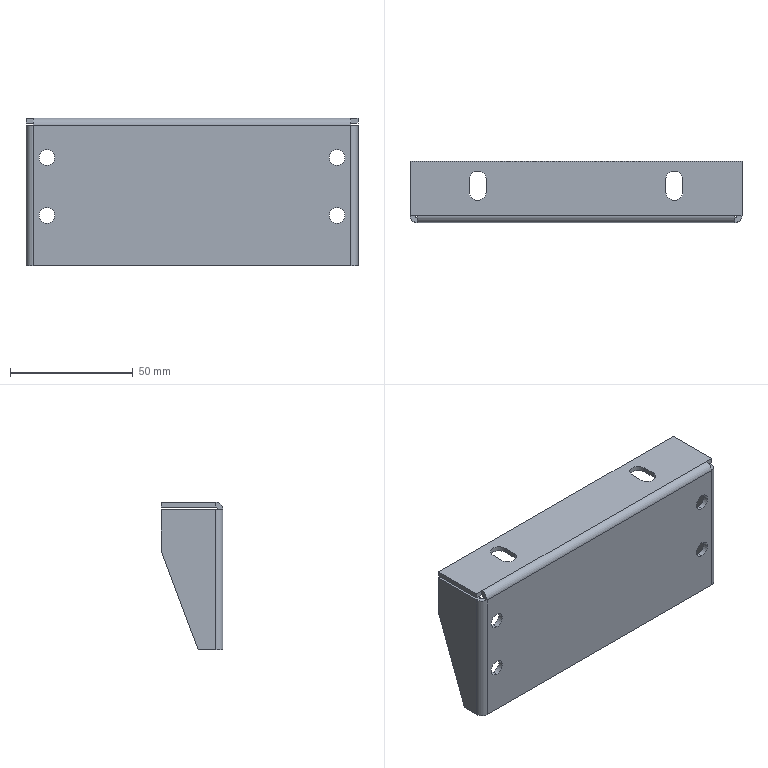Part | SolidWorks | features ICE 5, SMBaseFlange 2, EdgeFlange 1, FlatPattern 1, LPattern 1, SheetMetal 1 | 1 solid | 50 faces | box 135 x 25 x 60 mm | volume 25438 mm3 | plane 32 | cylinder 18 | commonest cylinder face diameters 6.4 x8 7 x4 2 x3 6 x3
STEP:
#1=CARTESIAN_POINT('',(158.643,39.897,40.8));
#2=VERTEX_POINT('',#1);
#3=CARTESIAN_POINT('',(158.643,39.897,47.2));
#4=VERTEX_POINT('',#3);
#5=CARTESIAN_POINT('',(158.643,39.897,44.));
#6=DIRECTION('',(0.,1.,0.));
#7=DIRECTION('',(0.,0.,1.));
#8=AXIS2_PLACEMENT_3D('',#5,#6,#7);
#9=CIRCLE('',#8,3.2);
#10=EDGE_CURVE('',#2,#4,#9,.T.);
#11=ORIENTED_EDGE('',*,*,#10,.T.);
#12=CARTESIAN_POINT('',(158.643,37.897,47.2));
#13=VERTEX_POINT('',#12);
#14=CARTESIAN_POINT('',(158.643,47.897,47.2));
#15=DIRECTION('',(0.,-1.,0.));
#16=VECTOR('',#15,1000.);
#17=LINE('',#14,#16);
#18=EDGE_CURVE('',#4,#13,#17,.T.);
#19=ORIENTED_EDGE('',*,*,#18,.T.);
#20=CARTESIAN_POINT('',(158.643,37.897,40.8));
#21=VERTEX_POINT('',#20);
#22=CARTESIAN_POINT('',(158.643,37.897,44.));
#23=DIRECTION('',(0.,-1.,0.));
#24=DIRECTION('',(0.,0.,-1.));
#25=AXIS2_PLACEMENT_3D('',#22,#23,#24);
#26=CIRCLE('',#25,3.2);
#27=EDGE_CURVE('',#13,#21,#26,.T.);
#28=ORIENTED_EDGE('',*,*,#27,.T.);
#29=CARTESIAN_POINT('',(158.643,47.897,40.8));
#30=DIRECTION('',(0.,-1.,0.));
#31=VECTOR('',#30,1000.);
#32=LINE('',#29,#31);
#33=EDGE_CURVE('',#2,#21,#32,.T.);
#34=ORIENTED_EDGE('',*,*,#33,.F.);
#35=EDGE_LOOP('',(#11,#19,#28,#34));
#36=FACE_OUTER_BOUND('',#35,.T.);
#37=CARTESIAN_POINT('',(158.643,47.897,44.));
#38=DIRECTION('',(0.,-1.,0.));
#39=DIRECTION('',(0.,0.,-1.));
#40=AXIS2_PLACEMENT_3D('',#37,#38,#39);
#41=CYLINDRICAL_SURFACE('',#40,3.2);
#42=ADVANCED_FACE('',(#36),#41,.F.);
#43=CARTESIAN_POINT('',(40.643,39.897,40.8));
#44=VERTEX_POINT('',#43);
#45=CARTESIAN_POINT('',(40.643,39.897,47.2));
#46=VERTEX_POINT('',#45);
#47=CARTESIAN_POINT('',(40.643,39.897,44.));
#48=DIRECTION('',(0.,1.,0.));
#49=DIRECTION('',(0.,0.,1.));
#50=AXIS2_PLACEMENT_3D('',#47,#48,#49);
#51=CIRCLE('',#50,3.2);
#52=EDGE_CURVE('',#44,#46,#51,.T.);
#53=ORIENTED_EDGE('',*,*,#52,.T.);
#54=CARTESIAN_POINT('',(40.643,37.897,47.2));
#55=VERTEX_POINT('',#54);
#56=CARTESIAN_POINT('',(40.643,47.897,47.2));
#57=DIRECTION('',(0.,-1.,0.));
#58=VECTOR('',#57,1000.);
#59=LINE('',#56,#58);
#60=EDGE_CURVE('',#46,#55,#59,.T.);
#61=ORIENTED_EDGE('',*,*,#60,.T.);
#62=CARTESIAN_POINT('',(40.643,37.897,40.8));
#63=VERTEX_POINT('',#62);
#64=CARTESIAN_POINT('',(40.643,37.897,44.));
#65=DIRECTION('',(0.,-1.,0.));
#66=DIRECTION('',(0.,0.,-1.));
#67=AXIS2_PLACEMENT_3D('',#64,#65,#66);
#68=CIRCLE('',#67,3.2);
#69=EDGE_CURVE('',#55,#63,#68,.T.);
#70=ORIENTED_EDGE('',*,*,#69,.T.);
#71=CARTESIAN_POINT('',(40.643,47.897,40.8));
#72=DIRECTION('',(0.,-1.,0.));
#73=VECTOR('',#72,1000.);
#74=LINE('',#71,#73);
#75=EDGE_CURVE('',#44,#63,#74,.T.);
#76=ORIENTED_EDGE('',*,*,#75,.F.);
#77=EDGE_LOOP('',(#53,#61,#70,#76));
#78=FACE_OUTER_BOUND('',#77,.T.);
#79=CARTESIAN_POINT('',(40.643,47.897,44.));
#80=DIRECTION('',(0.,-1.,0.));
#81=DIRECTION('',(0.,0.,-1.));
#82=AXIS2_PLACEMENT_3D('',#79,#80,#81);
#83=CYLINDRICAL_SURFACE('',#82,3.2);
#84=ADVANCED_FACE('',(#78),#83,.F.);
#85=CARTESIAN_POINT('',(40.643,39.897,17.3));
#86=VERTEX_POINT('',#85);
#87=CARTESIAN_POINT('',(40.643,39.897,23.7));
#88=VERTEX_POINT('',#87);
#89=CARTESIAN_POINT('',(40.643,39.897,20.5));
#90=DIRECTION('',(0.,1.,0.));
#91=DIRECTION('',(0.,0.,1.));
#92=AXIS2_PLACEMENT_3D('',#89,#90,#91);
#93=CIRCLE('',#92,3.2);
#94=EDGE_CURVE('',#86,#88,#93,.T.);
#95=ORIENTED_EDGE('',*,*,#94,.T.);
#96=CARTESIAN_POINT('',(40.643,37.897,23.7));
#97=VERTEX_POINT('',#96);
#98=CARTESIAN_POINT('',(40.643,47.897,23.7));
#99=DIRECTION('',(0.,-1.,0.));
#100=VECTOR('',#99,1000.);
#101=LINE('',#98,#100);
#102=EDGE_CURVE('',#88,#97,#101,.T.);
#103=ORIENTED_EDGE('',*,*,#102,.T.);
#104=CARTESIAN_POINT('',(40.643,37.897,17.3));
#105=VERTEX_POINT('',#104);
#106=CARTESIAN_POINT('',(40.643,37.897,20.5));
#107=DIRECTION('',(0.,-1.,0.));
#108=DIRECTION('',(0.,0.,-1.));
#109=AXIS2_PLACEMENT_3D('',#106,#107,#108);
#110=CIRCLE('',#109,3.2);
#111=EDGE_CURVE('',#97,#105,#110,.T.);
#112=ORIENTED_EDGE('',*,*,#111,.T.);
#113=CARTESIAN_POINT('',(40.643,47.897,17.3));
#114=DIRECTION('',(0.,-1.,0.));
#115=VECTOR('',#114,1000.);
#116=LINE('',#113,#115);
#117=EDGE_CURVE('',#86,#105,#116,.T.);
#118=ORIENTED_EDGE('',*,*,#117,.F.);
#119=EDGE_LOOP('',(#95,#103,#112,#118));
#120=FACE_OUTER_BOUND('',#119,.T.);
#121=CARTESIAN_POINT('',(40.643,47.897,20.5));
#122=DIRECTION('',(0.,-1.,0.));
#123=DIRECTION('',(0.,0.,-1.));
#124=AXIS2_PLACEMENT_3D('',#121,#122,#123);
#125=CYLINDRICAL_SURFACE('',#124,3.2);
#126=ADVANCED_FACE('',(#120),#125,.F.);
#127=CARTESIAN_POINT('',(158.643,39.897,17.3));
#128=VERTEX_POINT('',#127);
#129=CARTESIAN_POINT('',(158.643,39.897,23.7));
#130=VERTEX_POINT('',#129);
#131=CARTESIAN_POINT('',(158.643,39.897,20.5));
#132=DIRECTION('',(0.,1.,0.));
#133=DIRECTION('',(0.,0.,1.));
#134=AXIS2_PLACEMENT_3D('',#131,#132,#133);
#135=CIRCLE('',#134,3.2);
#136=EDGE_CURVE('',#128,#130,#135,.T.);
#137=ORIENTED_EDGE('',*,*,#136,.T.);
#138=CARTESIAN_POINT('',(158.643,37.897,23.7));
#139=VERTEX_POINT('',#138);
#140=CARTESIAN_POINT('',(158.643,47.897,23.7));
#141=DIRECTION('',(0.,-1.,0.));
#142=VECTOR('',#141,1000.);
#143=LINE('',#140,#142);
#144=EDGE_CURVE('',#130,#139,#143,.T.);
#145=ORIENTED_EDGE('',*,*,#144,.T.);
#146=CARTESIAN_POINT('',(158.643,37.897,17.3));
#147=VERTEX_POINT('',#146);
#148=CARTESIAN_POINT('',(158.643,37.897,20.5));
#149=DIRECTION('',(0.,-1.,0.));
#150=DIRECTION('',(0.,0.,-1.));
#151=AXIS2_PLACEMENT_3D('',#148,#149,#150);
#152=CIRCLE('',#151,3.2);
#153=EDGE_CURVE('',#139,#147,#152,.T.);
#154=ORIENTED_EDGE('',*,*,#153,.T.);
#155=CARTESIAN_POINT('',(158.643,47.897,17.3));
#156=DIRECTION('',(0.,-1.,0.));
#157=VECTOR('',#156,1000.);
#158=LINE('',#155,#157);
#159=EDGE_CURVE('',#128,#147,#158,.T.);
#160=ORIENTED_EDGE('',*,*,#159,.F.);
#161=EDGE_LOOP('',(#137,#145,#154,#160));
#162=FACE_OUTER_BOUND('',#161,.T.);
#163=CARTESIAN_POINT('',(158.643,47.897,20.5));
#164=DIRECTION('',(0.,-1.,0.));
#165=DIRECTION('',(0.,0.,-1.));
#166=AXIS2_PLACEMENT_3D('',#163,#164,#165);
#167=CYLINDRICAL_SURFACE('',#166,3.2);
#168=ADVANCED_FACE('',(#162),#167,.F.);
#169=CARTESIAN_POINT('',(34.143,62.897,57.));
#170=VERTEX_POINT('',#169);
#171=CARTESIAN_POINT('',(34.143,62.897,40.));
#172=VERTEX_POINT('',#171);
#173=CARTESIAN_POINT('',(34.143,62.897,60.));
#174=DIRECTION('',(0.,0.,-1.));
#175=VECTOR('',#174,1000.);
#176=LINE('',#173,#175);
#177=EDGE_CURVE('',#170,#172,#176,.T.);
#178=ORIENTED_EDGE('',*,*,#177,.F.);
#179=CARTESIAN_POINT('',(34.143,40.897,57.));
#180=VERTEX_POINT('',#179);
#181=CARTESIAN_POINT('',(34.143,62.897,57.));
#182=DIRECTION('',(0.,-1.,0.));
#183=VECTOR('',#182,1000.);
#184=LINE('',#181,#183);
#185=EDGE_CURVE('',#170,#180,#184,.T.);
#186=ORIENTED_EDGE('',*,*,#185,.T.);
#187=CARTESIAN_POINT('',(34.143,40.897,0.));
#188=VERTEX_POINT('',#187);
#189=CARTESIAN_POINT('',(34.143,40.897,60.));
#190=DIRECTION('',(0.,0.,-1.));
#191=VECTOR('',#190,1000.);
#192=LINE('',#189,#191);
#193=EDGE_CURVE('',#180,#188,#192,.T.);
#194=ORIENTED_EDGE('',*,*,#193,.T.);
#195=CARTESIAN_POINT('',(34.143,47.897,0.));
#196=VERTEX_POINT('',#195);
#197=CARTESIAN_POINT('',(34.143,62.897,0.));
#198=DIRECTION('',(0.,-1.,0.));
#199=VECTOR('',#198,1000.);
#200=LINE('',#197,#199);
#201=EDGE_CURVE('',#196,#188,#200,.T.);
#202=ORIENTED_EDGE('',*,*,#201,.F.);
#203=CARTESIAN_POINT('',(34.143,69.472,57.534));
#204=DIRECTION('',(0.,-0.3511,-0.9363));
#205=VECTOR('',#204,1000.);
#206=LINE('',#203,#205);
#207=EDGE_CURVE('',#172,#196,#206,.T.);
#208=ORIENTED_EDGE('',*,*,#207,.F.);
#209=EDGE_LOOP('',(#178,#186,#194,#202,#208));
#210=FACE_OUTER_BOUND('',#209,.T.);
#211=CARTESIAN_POINT('',(34.143,62.897,60.));
#212=DIRECTION('',(1.,0.,0.));
#213=DIRECTION('',(0.,0.,-1.));
#214=AXIS2_PLACEMENT_3D('',#211,#212,#213);
#215=PLANE('',#214);
#216=ADVANCED_FACE('',(#210),#215,.T.);
#217=CARTESIAN_POINT('',(32.143,62.897,57.));
#218=VERTEX_POINT('',#217);
#219=CARTESIAN_POINT('',(32.143,62.897,40.));
#220=VERTEX_POINT('',#219);
#221=CARTESIAN_POINT('',(32.143,62.897,60.));
#222=DIRECTION('',(0.,0.,-1.));
#223=VECTOR('',#222,1000.);
#224=LINE('',#221,#223);
#225=EDGE_CURVE('',#218,#220,#224,.T.);
#226=ORIENTED_EDGE('',*,*,#225,.F.);
#227=CARTESIAN_POINT('',(32.143,62.897,57.));
#228=DIRECTION('',(1.,0.,0.));
#229=VECTOR('',#228,1000.);
#230=LINE('',#227,#229);
#231=EDGE_CURVE('',#218,#170,#230,.T.);
#232=ORIENTED_EDGE('',*,*,#231,.T.);
#233=ORIENTED_EDGE('',*,*,#177,.T.);
#234=CARTESIAN_POINT('',(34.143,62.897,40.));
#235=DIRECTION('',(-1.,0.,0.));
#236=VECTOR('',#235,1000.);
#237=LINE('',#234,#236);
#238=EDGE_CURVE('',#172,#220,#237,.T.);
#239=ORIENTED_EDGE('',*,*,#238,.T.);
#240=EDGE_LOOP('',(#226,#232,#233,#239));
#241=FACE_OUTER_BOUND('',#240,.T.);
#242=CARTESIAN_POINT('',(32.143,62.897,60.));
#243=DIRECTION('',(0.,1.,0.));
#244=DIRECTION('',(0.,0.,1.));
#245=AXIS2_PLACEMENT_3D('',#242,#243,#244);
#246=PLANE('',#245);
#247=ADVANCED_FACE('',(#241),#246,.T.);
#248=CARTESIAN_POINT('',(32.143,40.897,57.));
#249=VERTEX_POINT('',#248);
#250=CARTESIAN_POINT('',(32.143,62.897,57.));
#251=DIRECTION('',(0.,-1.,0.));
#252=VECTOR('',#251,1000.);
#253=LINE('',#250,#252);
#254=EDGE_CURVE('',#218,#249,#253,.T.);
#255=ORIENTED_EDGE('',*,*,#254,.F.);
#256=ORIENTED_EDGE('',*,*,#225,.T.);
#257=CARTESIAN_POINT('',(32.143,47.897,0.));
#258=VERTEX_POINT('',#257);
#259=CARTESIAN_POINT('',(32.143,69.472,57.534));
#260=DIRECTION('',(0.,-0.3511,-0.9363));
#261=VECTOR('',#260,1000.);
#262=LINE('',#259,#261);
#263=EDGE_CURVE('',#220,#258,#262,.T.);
#264=ORIENTED_EDGE('',*,*,#263,.T.);
#265=CARTESIAN_POINT('',(32.143,40.897,0.));
#266=VERTEX_POINT('',#265);
#267=CARTESIAN_POINT('',(32.143,62.897,0.));
#268=DIRECTION('',(0.,-1.,0.));
#269=VECTOR('',#268,1000.);
#270=LINE('',#267,#269);
#271=EDGE_CURVE('',#258,#266,#270,.T.);
#272=ORIENTED_EDGE('',*,*,#271,.T.);
#273=CARTESIAN_POINT('',(32.143,40.897,60.));
#274=DIRECTION('',(0.,0.,-1.));
#275=VECTOR('',#274,1000.);
#276=LINE('',#273,#275);
#277=EDGE_CURVE('',#249,#266,#276,.T.);
#278=ORIENTED_EDGE('',*,*,#277,.F.);
#279=EDGE_LOOP('',(#255,#256,#264,#272,#278));
#280=FACE_OUTER_BOUND('',#279,.T.);
#281=CARTESIAN_POINT('',(32.143,62.897,60.));
#282=DIRECTION('',(1.,0.,0.));
#283=DIRECTION('',(0.,0.,-1.));
#284=AXIS2_PLACEMENT_3D('',#281,#282,#283);
#285=PLANE('',#284);
#286=ADVANCED_FACE('',(#280),#285,.F.);
#287=CARTESIAN_POINT('',(167.143,40.897,57.));
#288=VERTEX_POINT('',#287);
#289=CARTESIAN_POINT('',(167.143,62.897,57.));
#290=VERTEX_POINT('',#289);
#291=CARTESIAN_POINT('',(167.143,62.897,57.));
#292=DIRECTION('',(0.,1.,0.));
#293=VECTOR('',#292,1000.);
#294=LINE('',#291,#293);
#295=EDGE_CURVE('',#288,#290,#294,.T.);
#296=ORIENTED_EDGE('',*,*,#295,.F.);
#297=CARTESIAN_POINT('',(167.143,40.897,0.));
#298=VERTEX_POINT('',#297);
#299=CARTESIAN_POINT('',(167.143,40.897,60.));
#300=DIRECTION('',(0.,0.,-1.));
#301=VECTOR('',#300,1000.);
#302=LINE('',#299,#301);
#303=EDGE_CURVE('',#288,#298,#302,.T.);
#304=ORIENTED_EDGE('',*,*,#303,.T.);
#305=CARTESIAN_POINT('',(167.143,47.897,0.));
#306=VERTEX_POINT('',#305);
#307=CARTESIAN_POINT('',(167.143,37.897,0.));
#308=DIRECTION('',(0.,1.,0.));
#309=VECTOR('',#308,1000.);
#310=LINE('',#307,#309);
#311=EDGE_CURVE('',#298,#306,#310,.T.);
#312=ORIENTED_EDGE('',*,*,#311,.T.);
#313=CARTESIAN_POINT('',(167.143,62.897,40.));
#314=VERTEX_POINT('',#313);
#315=CARTESIAN_POINT('',(167.143,66.39,49.315));
#316=DIRECTION('',(0.,0.3511,0.9363));
#317=VECTOR('',#316,1000.);
#318=LINE('',#315,#317);
#319=EDGE_CURVE('',#306,#314,#318,.T.);
#320=ORIENTED_EDGE('',*,*,#319,.T.);
#321=CARTESIAN_POINT('',(167.143,62.897,60.));
#322=DIRECTION('',(0.,0.,-1.));
#323=VECTOR('',#322,1000.);
#324=LINE('',#321,#323);
#325=EDGE_CURVE('',#290,#314,#324,.T.);
#326=ORIENTED_EDGE('',*,*,#325,.F.);
#327=EDGE_LOOP('',(#296,#304,#312,#320,#326));
#328=FACE_OUTER_BOUND('',#327,.T.);
#329=CARTESIAN_POINT('',(167.143,37.897,60.));
#330=DIRECTION('',(-1.,0.,0.));
#331=DIRECTION('',(0.,0.,1.));
#332=AXIS2_PLACEMENT_3D('',#329,#330,#331);
#333=PLANE('',#332);
#334=ADVANCED_FACE('',(#328),#333,.F.);
#335=CARTESIAN_POINT('',(165.143,62.897,57.));
#336=VERTEX_POINT('',#335);
#337=CARTESIAN_POINT('',(165.143,62.897,40.));
#338=VERTEX_POINT('',#337);
#339=CARTESIAN_POINT('',(165.143,62.897,60.));
#340=DIRECTION('',(0.,0.,-1.));
#341=VECTOR('',#340,1000.);
#342=LINE('',#339,#341);
#343=EDGE_CURVE('',#336,#338,#342,.T.);
#344=ORIENTED_EDGE('',*,*,#343,.F.);
#345=CARTESIAN_POINT('',(167.143,62.897,57.));
#346=DIRECTION('',(-1.,0.,0.));
#347=VECTOR('',#346,1000.);
#348=LINE('',#345,#347);
#349=EDGE_CURVE('',#290,#336,#348,.T.);
#350=ORIENTED_EDGE('',*,*,#349,.F.);
#351=ORIENTED_EDGE('',*,*,#325,.T.);
#352=CARTESIAN_POINT('',(165.143,62.897,40.));
#353=DIRECTION('',(1.,0.,0.));
#354=VECTOR('',#353,1000.);
#355=LINE('',#352,#354);
#356=EDGE_CURVE('',#338,#314,#355,.T.);
#357=ORIENTED_EDGE('',*,*,#356,.F.);
#358=EDGE_LOOP('',(#344,#350,#351,#357));
#359=FACE_OUTER_BOUND('',#358,.T.);
#360=CARTESIAN_POINT('',(165.143,62.897,60.));
#361=DIRECTION('',(0.,1.,0.));
#362=DIRECTION('',(0.,0.,1.));
#363=AXIS2_PLACEMENT_3D('',#360,#361,#362);
#364=PLANE('',#363);
#365=ADVANCED_FACE('',(#359),#364,.T.);
#366=CARTESIAN_POINT('',(165.143,40.897,57.));
#367=VERTEX_POINT('',#366);
#368=CARTESIAN_POINT('',(165.143,40.897,0.));
#369=VERTEX_POINT('',#368);
#370=CARTESIAN_POINT('',(165.143,40.897,60.));
#371=DIRECTION('',(0.,0.,-1.));
#372=VECTOR('',#371,1000.);
#373=LINE('',#370,#372);
#374=EDGE_CURVE('',#367,#369,#373,.T.);
#375=ORIENTED_EDGE('',*,*,#374,.F.);
#376=CARTESIAN_POINT('',(165.143,37.897,57.));
#377=DIRECTION('',(0.,1.,0.));
#378=VECTOR('',#377,1000.);
#379=LINE('',#376,#378);
#380=EDGE_CURVE('',#367,#336,#379,.T.);
#381=ORIENTED_EDGE('',*,*,#380,.T.);
#382=ORIENTED_EDGE('',*,*,#343,.T.);
#383=CARTESIAN_POINT('',(165.143,47.897,0.));
#384=VERTEX_POINT('',#383);
#385=CARTESIAN_POINT('',(165.143,66.39,49.315));
#386=DIRECTION('',(0.,0.3511,0.9363));
#387=VECTOR('',#386,1000.);
#388=LINE('',#385,#387);
#389=EDGE_CURVE('',#384,#338,#388,.T.);
#390=ORIENTED_EDGE('',*,*,#389,.F.);
#391=CARTESIAN_POINT('',(165.143,37.897,0.));
#392=DIRECTION('',(0.,1.,0.));
#393=VECTOR('',#392,1000.);
#394=LINE('',#391,#393);
#395=EDGE_CURVE('',#369,#384,#394,.T.);
#396=ORIENTED_EDGE('',*,*,#395,.F.);
#397=EDGE_LOOP('',(#375,#381,#382,#390,#396));
#398=FACE_OUTER_BOUND('',#397,.T.);
#399=CARTESIAN_POINT('',(165.143,37.897,60.));
#400=DIRECTION('',(-1.,0.,0.));
#401=DIRECTION('',(0.,0.,1.));
#402=AXIS2_PLACEMENT_3D('',#399,#400,#401);
#403=PLANE('',#402);
#404=ADVANCED_FACE('',(#398),#403,.T.);
#405=ORIENTED_EDGE('',*,*,#144,.F.);
#406=CARTESIAN_POINT('',(158.643,39.897,20.5));
#407=DIRECTION('',(0.,1.,0.));
#408=DIRECTION('',(0.,0.,1.));
#409=AXIS2_PLACEMENT_3D('',#406,#407,#408);
#410=CIRCLE('',#409,3.2);
#411=EDGE_CURVE('',#130,#128,#410,.T.);
#412=ORIENTED_EDGE('',*,*,#411,.T.);
#413=ORIENTED_EDGE('',*,*,#159,.T.);
#414=CARTESIAN_POINT('',(158.643,37.897,20.5));
#415=DIRECTION('',(0.,-1.,0.));
#416=DIRECTION('',(0.,0.,-1.));
#417=AXIS2_PLACEMENT_3D('',#414,#415,#416);
#418=CIRCLE('',#417,3.2);
#419=EDGE_CURVE('',#147,#139,#418,.T.);
#420=ORIENTED_EDGE('',*,*,#419,.T.);
#421=EDGE_LOOP('',(#405,#412,#413,#420));
#422=FACE_OUTER_BOUND('',#421,.T.);
#423=CARTESIAN_POINT('',(158.643,47.897,20.5));
#424=DIRECTION('',(0.,-1.,0.));
#425=DIRECTION('',(0.,0.,-1.));
#426=AXIS2_PLACEMENT_3D('',#423,#424,#425);
#427=CYLINDRICAL_SURFACE('',#426,3.2);
#428=ADVANCED_FACE('',(#422),#427,.F.);
#429=ORIENTED_EDGE('',*,*,#102,.F.);
#430=CARTESIAN_POINT('',(40.643,39.897,20.5));
#431=DIRECTION('',(0.,1.,0.));
#432=DIRECTION('',(0.,0.,1.));
#433=AXIS2_PLACEMENT_3D('',#430,#431,#432);
#434=CIRCLE('',#433,3.2);
#435=EDGE_CURVE('',#88,#86,#434,.T.);
#436=ORIENTED_EDGE('',*,*,#435,.T.);
#437=ORIENTED_EDGE('',*,*,#117,.T.);
#438=CARTESIAN_POINT('',(40.643,37.897,20.5));
#439=DIRECTION('',(0.,-1.,0.));
#440=DIRECTION('',(0.,0.,-1.));
#441=AXIS2_PLACEMENT_3D('',#438,#439,#440);
#442=CIRCLE('',#441,3.2);
#443=EDGE_CURVE('',#105,#97,#442,.T.);
#444=ORIENTED_EDGE('',*,*,#443,.T.);
#445=EDGE_LOOP('',(#429,#436,#437,#444));
#446=FACE_OUTER_BOUND('',#445,.T.);
#447=CARTESIAN_POINT('',(40.643,47.897,20.5));
#448=DIRECTION('',(0.,-1.,0.));
#449=DIRECTION('',(0.,0.,-1.));
#450=AXIS2_PLACEMENT_3D('',#447,#448,#449);
#451=CYLINDRICAL_SURFACE('',#450,3.2);
#452=ADVANCED_FACE('',(#446),#451,.F.);
#453=ORIENTED_EDGE('',*,*,#395,.T.);
#454=CARTESIAN_POINT('',(165.143,47.897,0.));
#455=DIRECTION('',(1.,0.,0.));
#456=VECTOR('',#455,1000.);
#457=LINE('',#454,#456);
#458=EDGE_CURVE('',#384,#306,#457,.T.);
#459=ORIENTED_EDGE('',*,*,#458,.T.);
#460=ORIENTED_EDGE('',*,*,#311,.F.);
#461=CARTESIAN_POINT('',(167.143,40.897,0.));
#462=DIRECTION('',(-1.,0.,0.));
#463=VECTOR('',#462,1000.);
#464=LINE('',#461,#463);
#465=EDGE_CURVE('',#298,#369,#464,.T.);
#466=ORIENTED_EDGE('',*,*,#465,.T.);
#467=EDGE_LOOP('',(#453,#459,#460,#466));
#468=FACE_OUTER_BOUND('',#467,.T.);
#469=CARTESIAN_POINT('',(164.143,39.897,0.));
#470=DIRECTION('',(0.,0.,-1.));
#471=DIRECTION('',(-1.,0.,0.));
#472=AXIS2_PLACEMENT_3D('',#469,#470,#471);
#473=PLANE('',#472);
#474=ADVANCED_FACE('',(#468),#473,.T.);
#475=CARTESIAN_POINT('',(34.143,47.897,0.));
#476=DIRECTION('',(-1.,0.,0.));
#477=VECTOR('',#476,1000.);
#478=LINE('',#475,#477);
#479=EDGE_CURVE('',#196,#258,#478,.T.);
#480=ORIENTED_EDGE('',*,*,#479,.F.);
#481=ORIENTED_EDGE('',*,*,#201,.T.);
#482=CARTESIAN_POINT('',(34.143,40.897,0.));
#483=DIRECTION('',(-1.,0.,0.));
#484=VECTOR('',#483,1000.);
#485=LINE('',#482,#484);
#486=EDGE_CURVE('',#188,#266,#485,.T.);
#487=ORIENTED_EDGE('',*,*,#486,.T.);
#488=ORIENTED_EDGE('',*,*,#271,.F.);
#489=EDGE_LOOP('',(#480,#481,#487,#488));
#490=FACE_OUTER_BOUND('',#489,.T.);
#491=CARTESIAN_POINT('',(164.143,40.897,0.));
#492=DIRECTION('',(0.,0.,1.));
#493=DIRECTION('',(1.,0.,0.));
#494=AXIS2_PLACEMENT_3D('',#491,#492,#493);
#495=PLANE('',#494);
#496=ADVANCED_FACE('',(#490),#495,.F.);
#497=ORIENTED_EDGE('',*,*,#193,.F.);
#498=CARTESIAN_POINT('',(35.143,39.897,57.));
#499=VERTEX_POINT('',#498);
#500=CARTESIAN_POINT('',(35.143,40.897,57.));
#501=DIRECTION('',(0.,0.,1.));
#502=DIRECTION('',(0.,-1.,0.));
#503=AXIS2_PLACEMENT_3D('',#500,#501,#502);
#504=CIRCLE('',#503,1.);
#505=EDGE_CURVE('',#180,#499,#504,.T.);
#506=ORIENTED_EDGE('',*,*,#505,.T.);
#507=CARTESIAN_POINT('',(35.143,39.897,0.));
#508=VERTEX_POINT('',#507);
#509=CARTESIAN_POINT('',(35.143,39.897,60.));
#510=DIRECTION('',(0.,0.,-1.));
#511=VECTOR('',#510,1000.);
#512=LINE('',#509,#511);
#513=EDGE_CURVE('',#499,#508,#512,.T.);
#514=ORIENTED_EDGE('',*,*,#513,.T.);
#515=CARTESIAN_POINT('',(35.143,40.897,0.));
#516=DIRECTION('',(0.,0.,1.));
#517=DIRECTION('',(1.,0.,0.));
#518=AXIS2_PLACEMENT_3D('',#515,#516,#517);
#519=CIRCLE('',#518,1.);
#520=EDGE_CURVE('',#188,#508,#519,.T.);
#521=ORIENTED_EDGE('',*,*,#520,.F.);
#522=EDGE_LOOP('',(#497,#506,#514,#521));
#523=FACE_OUTER_BOUND('',#522,.T.);
#524=CARTESIAN_POINT('',(35.143,40.897,60.));
#525=DIRECTION('',(0.,0.,-1.));
#526=DIRECTION('',(-1.,0.,0.));
#527=AXIS2_PLACEMENT_3D('',#524,#525,#526);
#528=CYLINDRICAL_SURFACE('',#527,1.);
#529=ADVANCED_FACE('',(#523),#528,.F.);
#530=CARTESIAN_POINT('',(164.143,39.897,57.));
#531=VERTEX_POINT('',#530);
#532=CARTESIAN_POINT('',(164.143,39.897,0.));
#533=VERTEX_POINT('',#532);
#534=CARTESIAN_POINT('',(164.143,39.897,60.));
#535=DIRECTION('',(0.,0.,-1.));
#536=VECTOR('',#535,1000.);
#537=LINE('',#534,#536);
#538=EDGE_CURVE('',#531,#533,#537,.T.);
#539=ORIENTED_EDGE('',*,*,#538,.F.);
#540=CARTESIAN_POINT('',(164.143,40.897,57.));
#541=DIRECTION('',(0.,0.,1.));
#542=DIRECTION('',(0.,-1.,0.));
#543=AXIS2_PLACEMENT_3D('',#540,#541,#542);
#544=CIRCLE('',#543,1.);
#545=EDGE_CURVE('',#531,#367,#544,.T.);
#546=ORIENTED_EDGE('',*,*,#545,.T.);
#547=ORIENTED_EDGE('',*,*,#374,.T.);
#548=CARTESIAN_POINT('',(164.143,40.897,0.));
#549=DIRECTION('',(0.,0.,1.));
#550=DIRECTION('',(1.,0.,0.));
#551=AXIS2_PLACEMENT_3D('',#548,#549,#550);
#552=CIRCLE('',#551,1.);
#553=EDGE_CURVE('',#533,#369,#552,.T.);
#554=ORIENTED_EDGE('',*,*,#553,.F.);
#555=EDGE_LOOP('',(#539,#546,#547,#554));
#556=FACE_OUTER_BOUND('',#555,.T.);
#557=CARTESIAN_POINT('',(164.143,40.897,60.));
#558=DIRECTION('',(0.,0.,-1.));
#559=DIRECTION('',(-1.,0.,0.));
#560=AXIS2_PLACEMENT_3D('',#557,#558,#559);
#561=CYLINDRICAL_SURFACE('',#560,1.);
#562=ADVANCED_FACE('',(#556),#561,.F.);
#563=CARTESIAN_POINT('',(164.143,37.897,57.));
#564=VERTEX_POINT('',#563);
#565=CARTESIAN_POINT('',(164.143,40.897,57.));
#566=DIRECTION('',(0.,0.,1.));
#567=DIRECTION('',(0.,-1.,0.));
#568=AXIS2_PLACEMENT_3D('',#565,#566,#567);
#569=CIRCLE('',#568,3.);
#570=EDGE_CURVE('',#564,#288,#569,.T.);
#571=ORIENTED_EDGE('',*,*,#570,.T.);
#572=CARTESIAN_POINT('',(167.143,40.897,57.));
#573=DIRECTION('',(-1.,0.,0.));
#574=VECTOR('',#573,1000.);
#575=LINE('',#572,#574);
#576=EDGE_CURVE('',#288,#367,#575,.T.);
#577=ORIENTED_EDGE('',*,*,#576,.T.);
#578=ORIENTED_EDGE('',*,*,#545,.F.);
#579=CARTESIAN_POINT('',(164.143,39.897,57.));
#580=DIRECTION('',(0.,-1.,0.));
#581=VECTOR('',#580,1000.);
#582=LINE('',#579,#581);
#583=EDGE_CURVE('',#531,#564,#582,.T.);
#584=ORIENTED_EDGE('',*,*,#583,.T.);
#585=EDGE_LOOP('',(#571,#577,#578,#584));
#586=FACE_OUTER_BOUND('',#585,.T.);
#587=CARTESIAN_POINT('',(164.143,40.897,57.));
#588=DIRECTION('',(0.,0.,1.));
#589=DIRECTION('',(0.,-1.,0.));
#590=AXIS2_PLACEMENT_3D('',#587,#588,#589);
#591=PLANE('',#590);
#592=ADVANCED_FACE('',(#586),#591,.T.);
#593=ORIENTED_EDGE('',*,*,#10,.F.);
#594=CARTESIAN_POINT('',(158.643,39.897,44.));
#595=DIRECTION('',(0.,1.,0.));
#596=DIRECTION('',(0.,0.,1.));
#597=AXIS2_PLACEMENT_3D('',#594,#595,#596);
#598=CIRCLE('',#597,3.2);
#599=EDGE_CURVE('',#4,#2,#598,.T.);
#600=ORIENTED_EDGE('',*,*,#599,.F.);
#601=EDGE_LOOP('',(#593,#600));
#602=FACE_BOUND('',#601,.T.);
#603=ORIENTED_EDGE('',*,*,#52,.F.);
#604=CARTESIAN_POINT('',(40.643,39.897,44.));
#605=DIRECTION('',(0.,1.,0.));
#606=DIRECTION('',(0.,0.,1.));
#607=AXIS2_PLACEMENT_3D('',#604,#605,#606);
#608=CIRCLE('',#607,3.2);
#609=EDGE_CURVE('',#46,#44,#608,.T.);
#610=ORIENTED_EDGE('',*,*,#609,.F.);
#611=EDGE_LOOP('',(#603,#610));
#612=FACE_BOUND('',#611,.T.);
#613=ORIENTED_EDGE('',*,*,#513,.F.);
#614=CARTESIAN_POINT('',(164.143,39.897,57.));
#615=DIRECTION('',(-1.,0.,0.));
#616=VECTOR('',#615,1000.);
#617=LINE('',#614,#616);
#618=EDGE_CURVE('',#531,#499,#617,.T.);
#619=ORIENTED_EDGE('',*,*,#618,.F.);
#620=ORIENTED_EDGE('',*,*,#538,.T.);
#621=CARTESIAN_POINT('',(32.143,39.897,0.));
#622=DIRECTION('',(1.,0.,0.));
#623=VECTOR('',#622,1000.);
#624=LINE('',#621,#623);
#625=EDGE_CURVE('',#508,#533,#624,.T.);
#626=ORIENTED_EDGE('',*,*,#625,.F.);
#627=EDGE_LOOP('',(#613,#619,#620,#626));
#628=FACE_OUTER_BOUND('',#627,.T.);
#629=ORIENTED_EDGE('',*,*,#94,.F.);
#630=ORIENTED_EDGE('',*,*,#435,.F.);
#631=EDGE_LOOP('',(#629,#630));
#632=FACE_BOUND('',#631,.T.);
#633=ORIENTED_EDGE('',*,*,#136,.F.);
#634=ORIENTED_EDGE('',*,*,#411,.F.);
#635=EDGE_LOOP('',(#633,#634));
#636=FACE_BOUND('',#635,.T.);
#637=CARTESIAN_POINT('',(32.143,39.897,60.));
#638=DIRECTION('',(0.,1.,0.));
#639=DIRECTION('',(0.,0.,1.));
#640=AXIS2_PLACEMENT_3D('',#637,#638,#639);
#641=PLANE('',#640);
#642=ADVANCED_FACE('',(#602,#612,#628,#632,#636),#641,.T.);
#643=CARTESIAN_POINT('',(158.643,37.897,44.));
#644=DIRECTION('',(0.,-1.,0.));
#645=DIRECTION('',(0.,0.,-1.));
#646=AXIS2_PLACEMENT_3D('',#643,#644,#645);
#647=CIRCLE('',#646,3.2);
#648=EDGE_CURVE('',#21,#13,#647,.T.);
#649=ORIENTED_EDGE('',*,*,#648,.F.);
#650=ORIENTED_EDGE('',*,*,#27,.F.);
#651=EDGE_LOOP('',(#649,#650));
#652=FACE_BOUND('',#651,.T.);
#653=CARTESIAN_POINT('',(40.643,37.897,44.));
#654=DIRECTION('',(0.,-1.,0.));
#655=DIRECTION('',(0.,0.,-1.));
#656=AXIS2_PLACEMENT_3D('',#653,#654,#655);
#657=CIRCLE('',#656,3.2);
#658=EDGE_CURVE('',#63,#55,#657,.T.);
#659=ORIENTED_EDGE('',*,*,#658,.F.);
#660=ORIENTED_EDGE('',*,*,#69,.F.);
#661=EDGE_LOOP('',(#659,#660));
#662=FACE_BOUND('',#661,.T.);
#663=CARTESIAN_POINT('',(35.143,37.897,57.));
#664=VERTEX_POINT('',#663);
#665=CARTESIAN_POINT('',(164.143,37.897,57.));
#666=DIRECTION('',(-1.,0.,0.));
#667=VECTOR('',#666,1000.);
#668=LINE('',#665,#667);
#669=EDGE_CURVE('',#564,#664,#668,.T.);
#670=ORIENTED_EDGE('',*,*,#669,.T.);
#671=CARTESIAN_POINT('',(35.143,37.897,0.));
#672=VERTEX_POINT('',#671);
#673=CARTESIAN_POINT('',(35.143,37.897,60.));
#674=DIRECTION('',(0.,0.,-1.));
#675=VECTOR('',#674,1000.);
#676=LINE('',#673,#675);
#677=EDGE_CURVE('',#664,#672,#676,.T.);
#678=ORIENTED_EDGE('',*,*,#677,.T.);
#679=CARTESIAN_POINT('',(164.143,37.897,0.));
#680=VERTEX_POINT('',#679);
#681=CARTESIAN_POINT('',(32.143,37.897,0.));
#682=DIRECTION('',(1.,0.,0.));
#683=VECTOR('',#682,1000.);
#684=LINE('',#681,#683);
#685=EDGE_CURVE('',#672,#680,#684,.T.);
#686=ORIENTED_EDGE('',*,*,#685,.T.);
#687=CARTESIAN_POINT('',(164.143,37.897,60.));
#688=DIRECTION('',(0.,0.,-1.));
#689=VECTOR('',#688,1000.);
#690=LINE('',#687,#689);
#691=EDGE_CURVE('',#564,#680,#690,.T.);
#692=ORIENTED_EDGE('',*,*,#691,.F.);
#693=EDGE_LOOP('',(#670,#678,#686,#692));
#694=FACE_OUTER_BOUND('',#693,.T.);
#695=ORIENTED_EDGE('',*,*,#443,.F.);
#696=ORIENTED_EDGE('',*,*,#111,.F.);
#697=EDGE_LOOP('',(#695,#696));
#698=FACE_BOUND('',#697,.T.);
#699=ORIENTED_EDGE('',*,*,#419,.F.);
#700=ORIENTED_EDGE('',*,*,#153,.F.);
#701=EDGE_LOOP('',(#699,#700));
#702=FACE_BOUND('',#701,.T.);
#703=CARTESIAN_POINT('',(32.143,37.897,60.));
#704=DIRECTION('',(0.,1.,0.));
#705=DIRECTION('',(0.,0.,1.));
#706=AXIS2_PLACEMENT_3D('',#703,#704,#705);
#707=PLANE('',#706);
#708=ADVANCED_FACE('',(#652,#662,#694,#698,#702),#707,.F.);
#709=CARTESIAN_POINT('',(35.143,37.897,0.));
#710=DIRECTION('',(0.,1.,0.));
#711=VECTOR('',#710,1000.);
#712=LINE('',#709,#711);
#713=EDGE_CURVE('',#672,#508,#712,.T.);
#714=ORIENTED_EDGE('',*,*,#713,.F.);
#715=CARTESIAN_POINT('',(35.143,40.897,0.));
#716=DIRECTION('',(0.,0.,1.));
#717=DIRECTION('',(-1.,0.,0.));
#718=AXIS2_PLACEMENT_3D('',#715,#716,#717);
#719=CIRCLE('',#718,3.);
#720=EDGE_CURVE('',#266,#672,#719,.T.);
#721=ORIENTED_EDGE('',*,*,#720,.F.);
#722=ORIENTED_EDGE('',*,*,#486,.F.);
#723=ORIENTED_EDGE('',*,*,#520,.T.);
#724=EDGE_LOOP('',(#714,#721,#722,#723));
#725=FACE_OUTER_BOUND('',#724,.T.);
#726=CARTESIAN_POINT('',(35.143,37.897,0.));
#727=DIRECTION('',(0.,0.,-1.));
#728=DIRECTION('',(-1.,0.,0.));
#729=AXIS2_PLACEMENT_3D('',#726,#727,#728);
#730=PLANE('',#729);
#731=ADVANCED_FACE('',(#725),#730,.T.);
#732=ORIENTED_EDGE('',*,*,#685,.F.);
#733=ORIENTED_EDGE('',*,*,#713,.T.);
#734=ORIENTED_EDGE('',*,*,#625,.T.);
#735=CARTESIAN_POINT('',(164.143,39.897,0.));
#736=DIRECTION('',(0.,-1.,0.));
#737=VECTOR('',#736,1000.);
#738=LINE('',#735,#737);
#739=EDGE_CURVE('',#533,#680,#738,.T.);
#740=ORIENTED_EDGE('',*,*,#739,.T.);
#741=EDGE_LOOP('',(#732,#733,#734,#740));
#742=FACE_OUTER_BOUND('',#741,.T.);
#743=CARTESIAN_POINT('',(34.143,40.897,0.));
#744=DIRECTION('',(0.,0.,-1.));
#745=DIRECTION('',(-1.,0.,0.));
#746=AXIS2_PLACEMENT_3D('',#743,#744,#745);
#747=PLANE('',#746);
#748=ADVANCED_FACE('',(#742),#747,.T.);
#749=ORIENTED_EDGE('',*,*,#465,.F.);
#750=CARTESIAN_POINT('',(164.143,40.897,0.));
#751=DIRECTION('',(0.,0.,1.));
#752=DIRECTION('',(-1.,0.,0.));
#753=AXIS2_PLACEMENT_3D('',#750,#751,#752);
#754=CIRCLE('',#753,3.);
#755=EDGE_CURVE('',#680,#298,#754,.T.);
#756=ORIENTED_EDGE('',*,*,#755,.F.);
#757=ORIENTED_EDGE('',*,*,#739,.F.);
#758=ORIENTED_EDGE('',*,*,#553,.T.);
#759=EDGE_LOOP('',(#749,#756,#757,#758));
#760=FACE_OUTER_BOUND('',#759,.T.);
#761=CARTESIAN_POINT('',(167.143,40.897,0.));
#762=DIRECTION('',(0.,0.,-1.));
#763=DIRECTION('',(-1.,0.,0.));
#764=AXIS2_PLACEMENT_3D('',#761,#762,#763);
#765=PLANE('',#764);
#766=ADVANCED_FACE('',(#760),#765,.T.);
#767=ORIENTED_EDGE('',*,*,#505,.F.);
#768=CARTESIAN_POINT('',(34.143,40.897,57.));
#769=DIRECTION('',(-1.,0.,0.));
#770=VECTOR('',#769,1000.);
#771=LINE('',#768,#770);
#772=EDGE_CURVE('',#180,#249,#771,.T.);
#773=ORIENTED_EDGE('',*,*,#772,.T.);
#774=CARTESIAN_POINT('',(35.143,40.897,57.));
#775=DIRECTION('',(0.,0.,1.));
#776=DIRECTION('',(0.,-1.,0.));
#777=AXIS2_PLACEMENT_3D('',#774,#775,#776);
#778=CIRCLE('',#777,3.);
#779=EDGE_CURVE('',#249,#664,#778,.T.);
#780=ORIENTED_EDGE('',*,*,#779,.T.);
#781=CARTESIAN_POINT('',(35.143,39.897,57.));
#782=DIRECTION('',(0.,-1.,0.));
#783=VECTOR('',#782,1000.);
#784=LINE('',#781,#783);
#785=EDGE_CURVE('',#499,#664,#784,.T.);
#786=ORIENTED_EDGE('',*,*,#785,.F.);
#787=EDGE_LOOP('',(#767,#773,#780,#786));
#788=FACE_OUTER_BOUND('',#787,.T.);
#789=CARTESIAN_POINT('',(35.143,40.897,57.));
#790=DIRECTION('',(0.,0.,1.));
#791=DIRECTION('',(0.,-1.,0.));
#792=AXIS2_PLACEMENT_3D('',#789,#790,#791);
#793=PLANE('',#792);
#794=ADVANCED_FACE('',(#788),#793,.T.);
#795=ORIENTED_EDGE('',*,*,#779,.F.);
#796=ORIENTED_EDGE('',*,*,#277,.T.);
#797=ORIENTED_EDGE('',*,*,#720,.T.);
#798=ORIENTED_EDGE('',*,*,#677,.F.);
#799=EDGE_LOOP('',(#795,#796,#797,#798));
#800=FACE_OUTER_BOUND('',#799,.T.);
#801=CARTESIAN_POINT('',(35.143,40.897,60.));
#802=DIRECTION('',(0.,0.,-1.));
#803=DIRECTION('',(-1.,0.,0.));
#804=AXIS2_PLACEMENT_3D('',#801,#802,#803);
#805=CYLINDRICAL_SURFACE('',#804,3.);
#806=ADVANCED_FACE('',(#800),#805,.T.);
#807=ORIENTED_EDGE('',*,*,#570,.F.);
#808=ORIENTED_EDGE('',*,*,#691,.T.);
#809=ORIENTED_EDGE('',*,*,#755,.T.);
#810=ORIENTED_EDGE('',*,*,#303,.F.);
#811=EDGE_LOOP('',(#807,#808,#809,#810));
#812=FACE_OUTER_BOUND('',#811,.T.);
#813=CARTESIAN_POINT('',(164.143,40.897,60.));
#814=DIRECTION('',(0.,0.,-1.));
#815=DIRECTION('',(-1.,0.,0.));
#816=AXIS2_PLACEMENT_3D('',#813,#814,#815);
#817=CYLINDRICAL_SURFACE('',#816,3.);
#818=ADVANCED_FACE('',(#812),#817,.T.);
#819=CARTESIAN_POINT('',(35.143,40.897,58.));
#820=VERTEX_POINT('',#819);
#821=CARTESIAN_POINT('',(35.143,40.897,60.));
#822=VERTEX_POINT('',#821);
#823=CARTESIAN_POINT('',(35.143,40.897,60.));
#824=DIRECTION('',(0.,0.,1.));
#825=VECTOR('',#824,1000.);
#826=LINE('',#823,#825);
#827=EDGE_CURVE('',#820,#822,#826,.T.);
#828=ORIENTED_EDGE('',*,*,#827,.F.);
#829=CARTESIAN_POINT('',(35.143,40.897,57.));
#830=DIRECTION('',(-1.,0.,0.));
#831=DIRECTION('',(0.,0.,-1.));
#832=AXIS2_PLACEMENT_3D('',#829,#830,#831);
#833=CIRCLE('',#832,1.);
#834=EDGE_CURVE('',#499,#820,#833,.T.);
#835=ORIENTED_EDGE('',*,*,#834,.F.);
#836=ORIENTED_EDGE('',*,*,#785,.T.);
#837=CARTESIAN_POINT('',(35.143,40.897,57.));
#838=DIRECTION('',(-1.,0.,0.));
#839=DIRECTION('',(0.,0.,-1.));
#840=AXIS2_PLACEMENT_3D('',#837,#838,#839);
#841=CIRCLE('',#840,3.);
#842=EDGE_CURVE('',#664,#822,#841,.T.);
#843=ORIENTED_EDGE('',*,*,#842,.T.);
#844=EDGE_LOOP('',(#828,#835,#836,#843));
#845=FACE_OUTER_BOUND('',#844,.T.);
#846=CARTESIAN_POINT('',(35.143,40.897,57.));
#847=DIRECTION('',(-1.,0.,0.));
#848=DIRECTION('',(0.,0.,1.));
#849=AXIS2_PLACEMENT_3D('',#846,#847,#848);
#850=PLANE('',#849);
#851=ADVANCED_FACE('',(#845),#850,.T.);
#852=CARTESIAN_POINT('',(164.143,40.897,58.));
#853=VERTEX_POINT('',#852);
#854=CARTESIAN_POINT('',(164.143,40.897,57.));
#855=DIRECTION('',(1.,0.,0.));
#856=DIRECTION('',(0.,0.,-1.));
#857=AXIS2_PLACEMENT_3D('',#854,#855,#856);
#858=CIRCLE('',#857,1.);
#859=EDGE_CURVE('',#853,#531,#858,.T.);
#860=ORIENTED_EDGE('',*,*,#859,.F.);
#861=CARTESIAN_POINT('',(164.143,40.897,60.));
#862=VERTEX_POINT('',#861);
#863=CARTESIAN_POINT('',(164.143,40.897,58.));
#864=DIRECTION('',(0.,0.,1.));
#865=VECTOR('',#864,1000.);
#866=LINE('',#863,#865);
#867=EDGE_CURVE('',#853,#862,#866,.T.);
#868=ORIENTED_EDGE('',*,*,#867,.T.);
#869=CARTESIAN_POINT('',(164.143,40.897,57.));
#870=DIRECTION('',(1.,0.,0.));
#871=DIRECTION('',(0.,0.,-1.));
#872=AXIS2_PLACEMENT_3D('',#869,#870,#871);
#873=CIRCLE('',#872,3.);
#874=EDGE_CURVE('',#862,#564,#873,.T.);
#875=ORIENTED_EDGE('',*,*,#874,.T.);
#876=ORIENTED_EDGE('',*,*,#583,.F.);
#877=EDGE_LOOP('',(#860,#868,#875,#876));
#878=FACE_OUTER_BOUND('',#877,.T.);
#879=CARTESIAN_POINT('',(164.143,40.897,57.));
#880=DIRECTION('',(-1.,0.,0.));
#881=DIRECTION('',(0.,0.,1.));
#882=AXIS2_PLACEMENT_3D('',#879,#880,#881);
#883=PLANE('',#882);
#884=ADVANCED_FACE('',(#878),#883,.F.);
#885=ORIENTED_EDGE('',*,*,#669,.F.);
#886=ORIENTED_EDGE('',*,*,#874,.F.);
#887=CARTESIAN_POINT('',(0.,40.897,60.));
#888=DIRECTION('',(1.,0.,0.));
#889=VECTOR('',#888,1000.);
#890=LINE('',#887,#889);
#891=EDGE_CURVE('',#822,#862,#890,.T.);
#892=ORIENTED_EDGE('',*,*,#891,.F.);
#893=ORIENTED_EDGE('',*,*,#842,.F.);
#894=EDGE_LOOP('',(#885,#886,#892,#893));
#895=FACE_OUTER_BOUND('',#894,.T.);
#896=CARTESIAN_POINT('',(164.143,40.897,57.));
#897=DIRECTION('',(1.,0.,0.));
#898=DIRECTION('',(0.,0.,1.));
#899=AXIS2_PLACEMENT_3D('',#896,#897,#898);
#900=CYLINDRICAL_SURFACE('',#899,3.);
#901=ADVANCED_FACE('',(#895),#900,.T.);
#902=ORIENTED_EDGE('',*,*,#618,.T.);
#903=ORIENTED_EDGE('',*,*,#834,.T.);
#904=CARTESIAN_POINT('',(35.143,40.897,58.));
#905=DIRECTION('',(1.,0.,0.));
#906=VECTOR('',#905,1000.);
#907=LINE('',#904,#906);
#908=EDGE_CURVE('',#820,#853,#907,.T.);
#909=ORIENTED_EDGE('',*,*,#908,.T.);
#910=ORIENTED_EDGE('',*,*,#859,.T.);
#911=EDGE_LOOP('',(#902,#903,#909,#910));
#912=FACE_OUTER_BOUND('',#911,.T.);
#913=CARTESIAN_POINT('',(164.143,40.897,57.));
#914=DIRECTION('',(1.,0.,0.));
#915=DIRECTION('',(0.,0.,1.));
#916=AXIS2_PLACEMENT_3D('',#913,#914,#915);
#917=CYLINDRICAL_SURFACE('',#916,1.);
#918=ADVANCED_FACE('',(#912),#917,.F.);
#919=CARTESIAN_POINT('',(143.143,55.397,60.));
#920=VERTEX_POINT('',#919);
#921=CARTESIAN_POINT('',(136.143,55.397,60.));
#922=VERTEX_POINT('',#921);
#923=CARTESIAN_POINT('',(139.643,55.397,60.));
#924=DIRECTION('',(0.,0.,1.));
#925=DIRECTION('',(1.,0.,0.));
#926=AXIS2_PLACEMENT_3D('',#923,#924,#925);
#927=CIRCLE('',#926,3.5);
#928=EDGE_CURVE('',#920,#922,#927,.T.);
#929=ORIENTED_EDGE('',*,*,#928,.F.);
#930=CARTESIAN_POINT('',(143.143,50.397,60.));
#931=VERTEX_POINT('',#930);
#932=CARTESIAN_POINT('',(143.143,55.397,60.));
#933=DIRECTION('',(0.,1.,0.));
#934=VECTOR('',#933,1000.);
#935=LINE('',#932,#934);
#936=EDGE_CURVE('',#931,#920,#935,.T.);
#937=ORIENTED_EDGE('',*,*,#936,.F.);
#938=CARTESIAN_POINT('',(136.143,50.397,60.));
#939=VERTEX_POINT('',#938);
#940=CARTESIAN_POINT('',(139.643,50.397,60.));
#941=DIRECTION('',(0.,0.,1.));
#942=DIRECTION('',(1.,0.,0.));
#943=AXIS2_PLACEMENT_3D('',#940,#941,#942);
#944=CIRCLE('',#943,3.5);
#945=EDGE_CURVE('',#939,#931,#944,.T.);
#946=ORIENTED_EDGE('',*,*,#945,.F.);
#947=CARTESIAN_POINT('',(136.143,55.397,60.));
#948=DIRECTION('',(0.,-1.,0.));
#949=VECTOR('',#948,1000.);
#950=LINE('',#947,#949);
#951=EDGE_CURVE('',#922,#939,#950,.T.);
#952=ORIENTED_EDGE('',*,*,#951,.F.);
#953=EDGE_LOOP('',(#929,#937,#946,#952));
#954=FACE_BOUND('',#953,.T.);
#955=CARTESIAN_POINT('',(63.143,55.397,60.));
#956=VERTEX_POINT('',#955);
#957=CARTESIAN_POINT('',(56.143,55.397,60.));
#958=VERTEX_POINT('',#957);
#959=CARTESIAN_POINT('',(59.643,55.397,60.));
#960=DIRECTION('',(0.,0.,1.));
#961=DIRECTION('',(1.,0.,0.));
#962=AXIS2_PLACEMENT_3D('',#959,#960,#961);
#963=CIRCLE('',#962,3.5);
#964=EDGE_CURVE('',#956,#958,#963,.T.);
#965=ORIENTED_EDGE('',*,*,#964,.F.);
#966=CARTESIAN_POINT('',(63.143,50.397,60.));
#967=VERTEX_POINT('',#966);
#968=CARTESIAN_POINT('',(63.143,55.397,60.));
#969=DIRECTION('',(0.,1.,0.));
#970=VECTOR('',#969,1000.);
#971=LINE('',#968,#970);
#972=EDGE_CURVE('',#967,#956,#971,.T.);
#973=ORIENTED_EDGE('',*,*,#972,.F.);
#974=CARTESIAN_POINT('',(56.143,50.397,60.));
#975=VERTEX_POINT('',#974);
#976=CARTESIAN_POINT('',(59.643,50.397,60.));
#977=DIRECTION('',(0.,0.,1.));
#978=DIRECTION('',(1.,0.,0.));
#979=AXIS2_PLACEMENT_3D('',#976,#977,#978);
#980=CIRCLE('',#979,3.5);
#981=EDGE_CURVE('',#975,#967,#980,.T.);
#982=ORIENTED_EDGE('',*,*,#981,.F.);
#983=CARTESIAN_POINT('',(56.143,55.397,60.));
#984=DIRECTION('',(0.,-1.,0.));
#985=VECTOR('',#984,1000.);
#986=LINE('',#983,#985);
#987=EDGE_CURVE('',#958,#975,#986,.T.);
#988=ORIENTED_EDGE('',*,*,#987,.F.);
#989=EDGE_LOOP('',(#965,#973,#982,#988));
#990=FACE_BOUND('',#989,.T.);
#991=CARTESIAN_POINT('',(32.143,62.897,60.));
#992=VERTEX_POINT('',#991);
#993=CARTESIAN_POINT('',(167.143,62.897,60.));
#994=VERTEX_POINT('',#993);
#995=CARTESIAN_POINT('',(164.143,62.897,60.));
#996=DIRECTION('',(1.,0.,0.));
#997=VECTOR('',#996,1000.);
#998=LINE('',#995,#997);
#999=EDGE_CURVE('',#992,#994,#998,.T.);
#1000=ORIENTED_EDGE('',*,*,#999,.F.);
#1001=CARTESIAN_POINT('',(32.143,40.897,60.));
#1002=VERTEX_POINT('',#1001);
#1003=CARTESIAN_POINT('',(32.143,62.897,60.));
#1004=DIRECTION('',(0.,-1.,0.));
#1005=VECTOR('',#1004,1000.);
#1006=LINE('',#1003,#1005);
#1007=EDGE_CURVE('',#992,#1002,#1006,.T.);
#1008=ORIENTED_EDGE('',*,*,#1007,.T.);
#1009=CARTESIAN_POINT('',(35.143,40.897,60.));
#1010=DIRECTION('',(1.,0.,0.));
#1011=VECTOR('',#1010,1000.);
#1012=LINE('',#1009,#1011);
#1013=EDGE_CURVE('',#1002,#822,#1012,.T.);
#1014=ORIENTED_EDGE('',*,*,#1013,.T.);
#1015=ORIENTED_EDGE('',*,*,#891,.T.);
#1016=CARTESIAN_POINT('',(167.143,40.897,60.));
#1017=VERTEX_POINT('',#1016);
#1018=CARTESIAN_POINT('',(164.143,40.897,60.));
#1019=DIRECTION('',(1.,0.,0.));
#1020=VECTOR('',#1019,1000.);
#1021=LINE('',#1018,#1020);
#1022=EDGE_CURVE('',#862,#1017,#1021,.T.);
#1023=ORIENTED_EDGE('',*,*,#1022,.T.);
#1024=CARTESIAN_POINT('',(167.143,62.897,60.));
#1025=DIRECTION('',(0.,1.,0.));
#1026=VECTOR('',#1025,1000.);
#1027=LINE('',#1024,#1026);
#1028=EDGE_CURVE('',#1017,#994,#1027,.T.);
#1029=ORIENTED_EDGE('',*,*,#1028,.T.);
#1030=EDGE_LOOP('',(#1000,#1008,#1014,#1015,#1023,#1029));
#1031=FACE_OUTER_BOUND('',#1030,.T.);
#1032=CARTESIAN_POINT('',(0.,0.,60.));
#1033=DIRECTION('',(0.,0.,1.));
#1034=DIRECTION('',(0.,-1.,0.));
#1035=AXIS2_PLACEMENT_3D('',#1032,#1033,#1034);
#1036=PLANE('',#1035);
#1037=ADVANCED_FACE('',(#954,#990,#1031),#1036,.T.);
#1038=CARTESIAN_POINT('',(143.143,50.397,58.));
#1039=VERTEX_POINT('',#1038);
#1040=CARTESIAN_POINT('',(143.143,55.397,58.));
#1041=VERTEX_POINT('',#1040);
#1042=CARTESIAN_POINT('',(143.143,0.,58.));
#1043=DIRECTION('',(0.,1.,0.));
#1044=VECTOR('',#1043,1000.);
#1045=LINE('',#1042,#1044);
#1046=EDGE_CURVE('',#1039,#1041,#1045,.T.);
#1047=ORIENTED_EDGE('',*,*,#1046,.T.);
#1048=CARTESIAN_POINT('',(136.143,55.397,58.));
#1049=VERTEX_POINT('',#1048);
#1050=CARTESIAN_POINT('',(139.643,55.397,58.));
#1051=DIRECTION('',(0.,0.,1.));
#1052=DIRECTION('',(0.,-1.,0.));
#1053=AXIS2_PLACEMENT_3D('',#1050,#1051,#1052);
#1054=CIRCLE('',#1053,3.5);
#1055=EDGE_CURVE('',#1041,#1049,#1054,.T.);
#1056=ORIENTED_EDGE('',*,*,#1055,.T.);
#1057=CARTESIAN_POINT('',(136.143,50.397,58.));
#1058=VERTEX_POINT('',#1057);
#1059=CARTESIAN_POINT('',(136.143,0.,58.));
#1060=DIRECTION('',(0.,-1.,0.));
#1061=VECTOR('',#1060,1000.);
#1062=LINE('',#1059,#1061);
#1063=EDGE_CURVE('',#1049,#1058,#1062,.T.);
#1064=ORIENTED_EDGE('',*,*,#1063,.T.);
#1065=CARTESIAN_POINT('',(139.643,50.397,58.));
#1066=DIRECTION('',(0.,0.,1.));
#1067=DIRECTION('',(0.,-1.,0.));
#1068=AXIS2_PLACEMENT_3D('',#1065,#1066,#1067);
#1069=CIRCLE('',#1068,3.5);
#1070=EDGE_CURVE('',#1058,#1039,#1069,.T.);
#1071=ORIENTED_EDGE('',*,*,#1070,.T.);
#1072=EDGE_LOOP('',(#1047,#1056,#1064,#1071));
#1073=FACE_BOUND('',#1072,.T.);
#1074=CARTESIAN_POINT('',(63.143,50.397,58.));
#1075=VERTEX_POINT('',#1074);
#1076=CARTESIAN_POINT('',(63.143,55.397,58.));
#1077=VERTEX_POINT('',#1076);
#1078=CARTESIAN_POINT('',(63.143,0.,58.));
#1079=DIRECTION('',(0.,1.,0.));
#1080=VECTOR('',#1079,1000.);
#1081=LINE('',#1078,#1080);
#1082=EDGE_CURVE('',#1075,#1077,#1081,.T.);
#1083=ORIENTED_EDGE('',*,*,#1082,.T.);
#1084=CARTESIAN_POINT('',(56.143,55.397,58.));
#1085=VERTEX_POINT('',#1084);
#1086=CARTESIAN_POINT('',(59.643,55.397,58.));
#1087=DIRECTION('',(0.,0.,1.));
#1088=DIRECTION('',(0.,-1.,0.));
#1089=AXIS2_PLACEMENT_3D('',#1086,#1087,#1088);
#1090=CIRCLE('',#1089,3.5);
#1091=EDGE_CURVE('',#1077,#1085,#1090,.T.);
#1092=ORIENTED_EDGE('',*,*,#1091,.T.);
#1093=CARTESIAN_POINT('',(56.143,50.397,58.));
#1094=VERTEX_POINT('',#1093);
#1095=CARTESIAN_POINT('',(56.143,0.,58.));
#1096=DIRECTION('',(0.,-1.,0.));
#1097=VECTOR('',#1096,1000.);
#1098=LINE('',#1095,#1097);
#1099=EDGE_CURVE('',#1085,#1094,#1098,.T.);
#1100=ORIENTED_EDGE('',*,*,#1099,.T.);
#1101=CARTESIAN_POINT('',(59.643,50.397,58.));
#1102=DIRECTION('',(0.,0.,1.));
#1103=DIRECTION('',(0.,-1.,0.));
#1104=AXIS2_PLACEMENT_3D('',#1101,#1102,#1103);
#1105=CIRCLE('',#1104,3.5);
#1106=EDGE_CURVE('',#1094,#1075,#1105,.T.);
#1107=ORIENTED_EDGE('',*,*,#1106,.T.);
#1108=EDGE_LOOP('',(#1083,#1092,#1100,#1107));
#1109=FACE_BOUND('',#1108,.T.);
#1110=ORIENTED_EDGE('',*,*,#908,.F.);
#1111=CARTESIAN_POINT('',(32.143,40.897,58.));
#1112=VERTEX_POINT('',#1111);
#1113=CARTESIAN_POINT('',(35.143,40.897,58.));
#1114=DIRECTION('',(1.,0.,0.));
#1115=VECTOR('',#1114,1000.);
#1116=LINE('',#1113,#1115);
#1117=EDGE_CURVE('',#1112,#820,#1116,.T.);
#1118=ORIENTED_EDGE('',*,*,#1117,.F.);
#1119=CARTESIAN_POINT('',(32.143,62.897,58.));
#1120=VERTEX_POINT('',#1119);
#1121=CARTESIAN_POINT('',(32.143,62.897,58.));
#1122=DIRECTION('',(0.,-1.,0.));
#1123=VECTOR('',#1122,1000.);
#1124=LINE('',#1121,#1123);
#1125=EDGE_CURVE('',#1120,#1112,#1124,.T.);
#1126=ORIENTED_EDGE('',*,*,#1125,.F.);
#1127=CARTESIAN_POINT('',(167.143,62.897,58.));
#1128=VERTEX_POINT('',#1127);
#1129=CARTESIAN_POINT('',(0.,62.897,58.));
#1130=DIRECTION('',(1.,0.,0.));
#1131=VECTOR('',#1130,1000.);
#1132=LINE('',#1129,#1131);
#1133=EDGE_CURVE('',#1120,#1128,#1132,.T.);
#1134=ORIENTED_EDGE('',*,*,#1133,.T.);
#1135=CARTESIAN_POINT('',(167.143,40.897,58.));
#1136=VERTEX_POINT('',#1135);
#1137=CARTESIAN_POINT('',(167.143,62.897,58.));
#1138=DIRECTION('',(0.,1.,0.));
#1139=VECTOR('',#1138,1000.);
#1140=LINE('',#1137,#1139);
#1141=EDGE_CURVE('',#1136,#1128,#1140,.T.);
#1142=ORIENTED_EDGE('',*,*,#1141,.F.);
#1143=CARTESIAN_POINT('',(164.143,40.897,58.));
#1144=DIRECTION('',(1.,0.,0.));
#1145=VECTOR('',#1144,1000.);
#1146=LINE('',#1143,#1145);
#1147=EDGE_CURVE('',#853,#1136,#1146,.T.);
#1148=ORIENTED_EDGE('',*,*,#1147,.F.);
#1149=EDGE_LOOP('',(#1110,#1118,#1126,#1134,#1142,#1148));
#1150=FACE_OUTER_BOUND('',#1149,.T.);
#1151=CARTESIAN_POINT('',(0.,0.,58.));
#1152=DIRECTION('',(0.,0.,1.));
#1153=DIRECTION('',(0.,-1.,0.));
#1154=AXIS2_PLACEMENT_3D('',#1151,#1152,#1153);
#1155=PLANE('',#1154);
#1156=ADVANCED_FACE('',(#1073,#1109,#1150),#1155,.F.);
#1157=ORIENTED_EDGE('',*,*,#1133,.F.);
#1158=CARTESIAN_POINT('',(32.143,62.897,58.));
#1159=DIRECTION('',(0.,0.,1.));
#1160=VECTOR('',#1159,1000.);
#1161=LINE('',#1158,#1160);
#1162=EDGE_CURVE('',#1120,#992,#1161,.T.);
#1163=ORIENTED_EDGE('',*,*,#1162,.T.);
#1164=ORIENTED_EDGE('',*,*,#999,.T.);
#1165=CARTESIAN_POINT('',(167.143,62.897,58.));
#1166=DIRECTION('',(0.,0.,1.));
#1167=VECTOR('',#1166,1000.);
#1168=LINE('',#1165,#1167);
#1169=EDGE_CURVE('',#1128,#994,#1168,.T.);
#1170=ORIENTED_EDGE('',*,*,#1169,.F.);
#1171=EDGE_LOOP('',(#1157,#1163,#1164,#1170));
#1172=FACE_OUTER_BOUND('',#1171,.T.);
#1173=CARTESIAN_POINT('',(164.143,62.897,60.));
#1174=DIRECTION('',(0.,1.,0.));
#1175=DIRECTION('',(0.,0.,1.));
#1176=AXIS2_PLACEMENT_3D('',#1173,#1174,#1175);
#1177=PLANE('',#1176);
#1178=ADVANCED_FACE('',(#1172),#1177,.T.);
#1179=ORIENTED_EDGE('',*,*,#207,.T.);
#1180=ORIENTED_EDGE('',*,*,#479,.T.);
#1181=ORIENTED_EDGE('',*,*,#263,.F.);
#1182=ORIENTED_EDGE('',*,*,#238,.F.);
#1183=EDGE_LOOP('',(#1179,#1180,#1181,#1182));
#1184=FACE_OUTER_BOUND('',#1183,.T.);
#1185=CARTESIAN_POINT('',(34.143,69.472,57.534));
#1186=DIRECTION('',(0.,-0.9363,0.3511));
#1187=DIRECTION('',(0.,-0.3511,-0.9363));
#1188=AXIS2_PLACEMENT_3D('',#1185,#1186,#1187);
#1189=PLANE('',#1188);
#1190=ADVANCED_FACE('',(#1184),#1189,.F.);
#1191=ORIENTED_EDGE('',*,*,#389,.T.);
#1192=ORIENTED_EDGE('',*,*,#356,.T.);
#1193=ORIENTED_EDGE('',*,*,#319,.F.);
#1194=ORIENTED_EDGE('',*,*,#458,.F.);
#1195=EDGE_LOOP('',(#1191,#1192,#1193,#1194));
#1196=FACE_OUTER_BOUND('',#1195,.T.);
#1197=CARTESIAN_POINT('',(165.143,66.39,49.315));
#1198=DIRECTION('',(0.,-0.9363,0.3511));
#1199=DIRECTION('',(0.,0.3511,0.9363));
#1200=AXIS2_PLACEMENT_3D('',#1197,#1198,#1199);
#1201=PLANE('',#1200);
#1202=ADVANCED_FACE('',(#1196),#1201,.F.);
#1203=CARTESIAN_POINT('',(63.143,55.397,-131.));
#1204=DIRECTION('',(0.,0.,1.));
#1205=VECTOR('',#1204,1000.);
#1206=LINE('',#1203,#1205);
#1207=EDGE_CURVE('',#1077,#956,#1206,.T.);
#1208=ORIENTED_EDGE('',*,*,#1207,.T.);
#1209=ORIENTED_EDGE('',*,*,#964,.T.);
#1210=CARTESIAN_POINT('',(56.143,55.397,-131.));
#1211=DIRECTION('',(0.,0.,1.));
#1212=VECTOR('',#1211,1000.);
#1213=LINE('',#1210,#1212);
#1214=EDGE_CURVE('',#1085,#958,#1213,.T.);
#1215=ORIENTED_EDGE('',*,*,#1214,.F.);
#1216=ORIENTED_EDGE('',*,*,#1091,.F.);
#1217=EDGE_LOOP('',(#1208,#1209,#1215,#1216));
#1218=FACE_OUTER_BOUND('',#1217,.T.);
#1219=CARTESIAN_POINT('',(59.643,55.397,-131.));
#1220=DIRECTION('',(0.,0.,1.));
#1221=DIRECTION('',(1.,0.,0.));
#1222=AXIS2_PLACEMENT_3D('',#1219,#1220,#1221);
#1223=CYLINDRICAL_SURFACE('',#1222,3.5);
#1224=ADVANCED_FACE('',(#1218),#1223,.F.);
#1225=CARTESIAN_POINT('',(63.143,50.397,-131.));
#1226=DIRECTION('',(0.,0.,1.));
#1227=VECTOR('',#1226,1000.);
#1228=LINE('',#1225,#1227);
#1229=EDGE_CURVE('',#1075,#967,#1228,.T.);
#1230=ORIENTED_EDGE('',*,*,#1229,.T.);
#1231=ORIENTED_EDGE('',*,*,#972,.T.);
#1232=ORIENTED_EDGE('',*,*,#1207,.F.);
#1233=ORIENTED_EDGE('',*,*,#1082,.F.);
#1234=EDGE_LOOP('',(#1230,#1231,#1232,#1233));
#1235=FACE_OUTER_BOUND('',#1234,.T.);
#1236=CARTESIAN_POINT('',(63.143,55.397,-131.));
#1237=DIRECTION('',(1.,0.,0.));
#1238=DIRECTION('',(0.,0.,-1.));
#1239=AXIS2_PLACEMENT_3D('',#1236,#1237,#1238);
#1240=PLANE('',#1239);
#1241=ADVANCED_FACE('',(#1235),#1240,.F.);
#1242=CARTESIAN_POINT('',(56.143,50.397,-131.));
#1243=DIRECTION('',(0.,0.,1.));
#1244=VECTOR('',#1243,1000.);
#1245=LINE('',#1242,#1244);
#1246=EDGE_CURVE('',#1094,#975,#1245,.T.);
#1247=ORIENTED_EDGE('',*,*,#1246,.T.);
#1248=ORIENTED_EDGE('',*,*,#981,.T.);
#1249=ORIENTED_EDGE('',*,*,#1229,.F.);
#1250=ORIENTED_EDGE('',*,*,#1106,.F.);
#1251=EDGE_LOOP('',(#1247,#1248,#1249,#1250));
#1252=FACE_OUTER_BOUND('',#1251,.T.);
#1253=CARTESIAN_POINT('',(59.643,50.397,-131.));
#1254=DIRECTION('',(0.,0.,1.));
#1255=DIRECTION('',(1.,0.,0.));
#1256=AXIS2_PLACEMENT_3D('',#1253,#1254,#1255);
#1257=CYLINDRICAL_SURFACE('',#1256,3.5);
#1258=ADVANCED_FACE('',(#1252),#1257,.F.);
#1259=ORIENTED_EDGE('',*,*,#1214,.T.);
#1260=ORIENTED_EDGE('',*,*,#987,.T.);
#1261=ORIENTED_EDGE('',*,*,#1246,.F.);
#1262=ORIENTED_EDGE('',*,*,#1099,.F.);
#1263=EDGE_LOOP('',(#1259,#1260,#1261,#1262));
#1264=FACE_OUTER_BOUND('',#1263,.T.);
#1265=CARTESIAN_POINT('',(56.143,55.397,-131.));
#1266=DIRECTION('',(-1.,0.,0.));
#1267=DIRECTION('',(0.,0.,1.));
#1268=AXIS2_PLACEMENT_3D('',#1265,#1266,#1267);
#1269=PLANE('',#1268);
#1270=ADVANCED_FACE('',(#1264),#1269,.F.);
#1271=CARTESIAN_POINT('',(143.143,55.397,-131.));
#1272=DIRECTION('',(0.,0.,1.));
#1273=VECTOR('',#1272,1000.);
#1274=LINE('',#1271,#1273);
#1275=EDGE_CURVE('',#1041,#920,#1274,.T.);
#1276=ORIENTED_EDGE('',*,*,#1275,.T.);
#1277=ORIENTED_EDGE('',*,*,#928,.T.);
#1278=CARTESIAN_POINT('',(136.143,55.397,-131.));
#1279=DIRECTION('',(0.,0.,1.));
#1280=VECTOR('',#1279,1000.);
#1281=LINE('',#1278,#1280);
#1282=EDGE_CURVE('',#1049,#922,#1281,.T.);
#1283=ORIENTED_EDGE('',*,*,#1282,.F.);
#1284=ORIENTED_EDGE('',*,*,#1055,.F.);
#1285=EDGE_LOOP('',(#1276,#1277,#1283,#1284));
#1286=FACE_OUTER_BOUND('',#1285,.T.);
#1287=CARTESIAN_POINT('',(139.643,55.397,-131.));
#1288=DIRECTION('',(0.,0.,1.));
#1289=DIRECTION('',(1.,0.,0.));
#1290=AXIS2_PLACEMENT_3D('',#1287,#1288,#1289);
#1291=CYLINDRICAL_SURFACE('',#1290,3.5);
#1292=ADVANCED_FACE('',(#1286),#1291,.F.);
#1293=CARTESIAN_POINT('',(143.143,50.397,-131.));
#1294=DIRECTION('',(0.,0.,1.));
#1295=VECTOR('',#1294,1000.);
#1296=LINE('',#1293,#1295);
#1297=EDGE_CURVE('',#1039,#931,#1296,.T.);
#1298=ORIENTED_EDGE('',*,*,#1297,.T.);
#1299=ORIENTED_EDGE('',*,*,#936,.T.);
#1300=ORIENTED_EDGE('',*,*,#1275,.F.);
#1301=ORIENTED_EDGE('',*,*,#1046,.F.);
#1302=EDGE_LOOP('',(#1298,#1299,#1300,#1301));
#1303=FACE_OUTER_BOUND('',#1302,.T.);
#1304=CARTESIAN_POINT('',(143.143,55.397,-131.));
#1305=DIRECTION('',(1.,0.,0.));
#1306=DIRECTION('',(0.,0.,-1.));
#1307=AXIS2_PLACEMENT_3D('',#1304,#1305,#1306);
#1308=PLANE('',#1307);
#1309=ADVANCED_FACE('',(#1303),#1308,.F.);
#1310=CARTESIAN_POINT('',(136.143,50.397,-131.));
#1311=DIRECTION('',(0.,0.,1.));
#1312=VECTOR('',#1311,1000.);
#1313=LINE('',#1310,#1312);
#1314=EDGE_CURVE('',#1058,#939,#1313,.T.);
#1315=ORIENTED_EDGE('',*,*,#1314,.T.);
#1316=ORIENTED_EDGE('',*,*,#945,.T.);
#1317=ORIENTED_EDGE('',*,*,#1297,.F.);
#1318=ORIENTED_EDGE('',*,*,#1070,.F.);
#1319=EDGE_LOOP('',(#1315,#1316,#1317,#1318));
#1320=FACE_OUTER_BOUND('',#1319,.T.);
#1321=CARTESIAN_POINT('',(139.643,50.397,-131.));
#1322=DIRECTION('',(0.,0.,1.));
#1323=DIRECTION('',(1.,0.,0.));
#1324=AXIS2_PLACEMENT_3D('',#1321,#1322,#1323);
#1325=CYLINDRICAL_SURFACE('',#1324,3.5);
#1326=ADVANCED_FACE('',(#1320),#1325,.F.);
#1327=ORIENTED_EDGE('',*,*,#1282,.T.);
#1328=ORIENTED_EDGE('',*,*,#951,.T.);
#1329=ORIENTED_EDGE('',*,*,#1314,.F.);
#1330=ORIENTED_EDGE('',*,*,#1063,.F.);
#1331=EDGE_LOOP('',(#1327,#1328,#1329,#1330));
#1332=FACE_OUTER_BOUND('',#1331,.T.);
#1333=CARTESIAN_POINT('',(136.143,55.397,-131.));
#1334=DIRECTION('',(-1.,0.,0.));
#1335=DIRECTION('',(0.,0.,1.));
#1336=AXIS2_PLACEMENT_3D('',#1333,#1334,#1335);
#1337=PLANE('',#1336);
#1338=ADVANCED_FACE('',(#1332),#1337,.F.);
#1339=ORIENTED_EDGE('',*,*,#60,.F.);
#1340=ORIENTED_EDGE('',*,*,#609,.T.);
#1341=ORIENTED_EDGE('',*,*,#75,.T.);
#1342=ORIENTED_EDGE('',*,*,#658,.T.);
#1343=EDGE_LOOP('',(#1339,#1340,#1341,#1342));
#1344=FACE_OUTER_BOUND('',#1343,.T.);
#1345=CARTESIAN_POINT('',(40.643,47.897,44.));
#1346=DIRECTION('',(0.,-1.,0.));
#1347=DIRECTION('',(0.,0.,-1.));
#1348=AXIS2_PLACEMENT_3D('',#1345,#1346,#1347);
#1349=CYLINDRICAL_SURFACE('',#1348,3.2);
#1350=ADVANCED_FACE('',(#1344),#1349,.F.);
#1351=ORIENTED_EDGE('',*,*,#18,.F.);
#1352=ORIENTED_EDGE('',*,*,#599,.T.);
#1353=ORIENTED_EDGE('',*,*,#33,.T.);
#1354=ORIENTED_EDGE('',*,*,#648,.T.);
#1355=EDGE_LOOP('',(#1351,#1352,#1353,#1354));
#1356=FACE_OUTER_BOUND('',#1355,.T.);
#1357=CARTESIAN_POINT('',(158.643,47.897,44.));
#1358=DIRECTION('',(0.,-1.,0.));
#1359=DIRECTION('',(0.,0.,-1.));
#1360=AXIS2_PLACEMENT_3D('',#1357,#1358,#1359);
#1361=CYLINDRICAL_SURFACE('',#1360,3.2);
#1362=ADVANCED_FACE('',(#1356),#1361,.F.);
#1363=ORIENTED_EDGE('',*,*,#576,.F.);
#1364=ORIENTED_EDGE('',*,*,#295,.T.);
#1365=ORIENTED_EDGE('',*,*,#349,.T.);
#1366=ORIENTED_EDGE('',*,*,#380,.F.);
#1367=EDGE_LOOP('',(#1363,#1364,#1365,#1366));
#1368=FACE_OUTER_BOUND('',#1367,.T.);
#1369=CARTESIAN_POINT('',(167.143,62.897,57.));
#1370=DIRECTION('',(0.,0.,1.));
#1371=DIRECTION('',(0.,1.,0.));
#1372=AXIS2_PLACEMENT_3D('',#1369,#1370,#1371);
#1373=PLANE('',#1372);
#1374=ADVANCED_FACE('',(#1368),#1373,.T.);
#1375=ORIENTED_EDGE('',*,*,#231,.F.);
#1376=ORIENTED_EDGE('',*,*,#254,.T.);
#1377=ORIENTED_EDGE('',*,*,#772,.F.);
#1378=ORIENTED_EDGE('',*,*,#185,.F.);
#1379=EDGE_LOOP('',(#1375,#1376,#1377,#1378));
#1380=FACE_OUTER_BOUND('',#1379,.T.);
#1381=CARTESIAN_POINT('',(32.143,62.897,57.));
#1382=DIRECTION('',(0.,0.,1.));
#1383=DIRECTION('',(0.,-1.,0.));
#1384=AXIS2_PLACEMENT_3D('',#1381,#1382,#1383);
#1385=PLANE('',#1384);
#1386=ADVANCED_FACE('',(#1380),#1385,.T.);
#1387=ORIENTED_EDGE('',*,*,#1013,.F.);
#1388=CARTESIAN_POINT('',(32.143,40.897,58.));
#1389=DIRECTION('',(0.,0.,1.));
#1390=VECTOR('',#1389,1000.);
#1391=LINE('',#1388,#1390);
#1392=EDGE_CURVE('',#1112,#1002,#1391,.T.);
#1393=ORIENTED_EDGE('',*,*,#1392,.F.);
#1394=ORIENTED_EDGE('',*,*,#1117,.T.);
#1395=ORIENTED_EDGE('',*,*,#827,.T.);
#1396=EDGE_LOOP('',(#1387,#1393,#1394,#1395));
#1397=FACE_OUTER_BOUND('',#1396,.T.);
#1398=CARTESIAN_POINT('',(35.143,40.897,58.));
#1399=DIRECTION('',(0.,-1.,0.));
#1400=DIRECTION('',(0.,0.,-1.));
#1401=AXIS2_PLACEMENT_3D('',#1398,#1399,#1400);
#1402=PLANE('',#1401);
#1403=ADVANCED_FACE('',(#1397),#1402,.T.);
#1404=ORIENTED_EDGE('',*,*,#1007,.F.);
#1405=ORIENTED_EDGE('',*,*,#1162,.F.);
#1406=ORIENTED_EDGE('',*,*,#1125,.T.);
#1407=ORIENTED_EDGE('',*,*,#1392,.T.);
#1408=EDGE_LOOP('',(#1404,#1405,#1406,#1407));
#1409=FACE_OUTER_BOUND('',#1408,.T.);
#1410=CARTESIAN_POINT('',(32.143,62.897,58.));
#1411=DIRECTION('',(-1.,0.,0.));
#1412=DIRECTION('',(0.,0.,1.));
#1413=AXIS2_PLACEMENT_3D('',#1410,#1411,#1412);
#1414=PLANE('',#1413);
#1415=ADVANCED_FACE('',(#1409),#1414,.T.);
#1416=ORIENTED_EDGE('',*,*,#1028,.F.);
#1417=CARTESIAN_POINT('',(167.143,40.897,58.));
#1418=DIRECTION('',(0.,0.,1.));
#1419=VECTOR('',#1418,1000.);
#1420=LINE('',#1417,#1419);
#1421=EDGE_CURVE('',#1136,#1017,#1420,.T.);
#1422=ORIENTED_EDGE('',*,*,#1421,.F.);
#1423=ORIENTED_EDGE('',*,*,#1141,.T.);
#1424=ORIENTED_EDGE('',*,*,#1169,.T.);
#1425=EDGE_LOOP('',(#1416,#1422,#1423,#1424));
#1426=FACE_OUTER_BOUND('',#1425,.T.);
#1427=CARTESIAN_POINT('',(167.143,62.897,58.));
#1428=DIRECTION('',(1.,0.,0.));
#1429=DIRECTION('',(0.,0.,-1.));
#1430=AXIS2_PLACEMENT_3D('',#1427,#1428,#1429);
#1431=PLANE('',#1430);
#1432=ADVANCED_FACE('',(#1426),#1431,.T.);
#1433=ORIENTED_EDGE('',*,*,#1022,.F.);
#1434=ORIENTED_EDGE('',*,*,#867,.F.);
#1435=ORIENTED_EDGE('',*,*,#1147,.T.);
#1436=ORIENTED_EDGE('',*,*,#1421,.T.);
#1437=EDGE_LOOP('',(#1433,#1434,#1435,#1436));
#1438=FACE_OUTER_BOUND('',#1437,.T.);
#1439=CARTESIAN_POINT('',(164.143,40.897,58.));
#1440=DIRECTION('',(0.,-1.,0.));
#1441=DIRECTION('',(0.,0.,-1.));
#1442=AXIS2_PLACEMENT_3D('',#1439,#1440,#1441);
#1443=PLANE('',#1442);
#1444=ADVANCED_FACE('',(#1438),#1443,.T.);
#1445=CLOSED_SHELL('',(#42,#84,#126,#168,#216,#247,#286,#334,#365,#404,#428,#452,#474,#496,#529,#562,#592,#642,#708,#731,#748,#766,#794,#806,#818,#851,#884,#901,#918,#1037,#1156,#1178,#1190,#1202,#1224,#1241,#1258,#1270,#1292,#1309,#1326,#1338,#1350,#1362,#1374,#1386,#1403,#1415,#1432,#1444));
#1446=MANIFOLD_SOLID_BREP('',#1445);
#1447=CARTESIAN_POINT('',(0.,0.,0.));
#1448=DIRECTION('',(0.,0.,1.));
#1449=DIRECTION('',(1.,0.,0.));
#1450=AXIS2_PLACEMENT_3D('',#1447,#1448,#1449);
#1451=(LENGTH_UNIT()NAMED_UNIT(*)SI_UNIT(.MILLI.,.METRE.));
#1452=UNCERTAINTY_MEASURE_WITH_UNIT(LENGTH_MEASURE(0.00001),#1451,'','');
#1453=(NAMED_UNIT(*)PLANE_ANGLE_UNIT()SI_UNIT($,.RADIAN.));
#1454=(NAMED_UNIT(*)SI_UNIT($,.STERADIAN.)SOLID_ANGLE_UNIT());
#1455=(GEOMETRIC_REPRESENTATION_CONTEXT(3)GLOBAL_UNCERTAINTY_ASSIGNED_CONTEXT((#1452))GLOBAL_UNIT_ASSIGNED_CONTEXT((#1451,#1453,#1454))REPRESENTATION_CONTEXT('',''));
#1456=ADVANCED_BREP_SHAPE_REPRESENTATION('',(#1446,#1450),#1455);